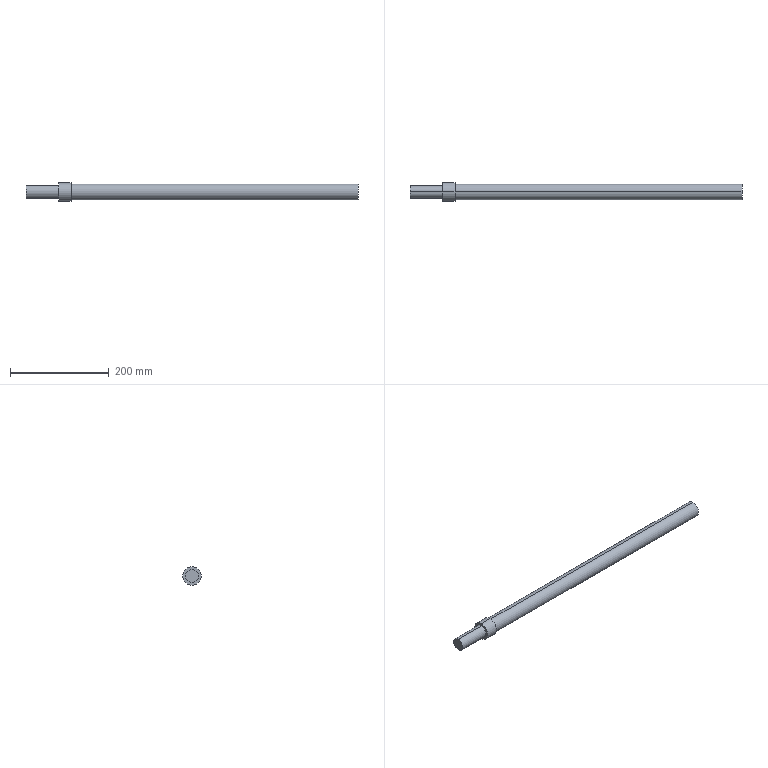Part | SolidWorks | features Revolution 1 | 1 solid | 10 faces | box 671 x 37 x 37 mm | volume 528385 mm3 | cylinder 6 | plane 4 | commonest cylinder face diameters 26 x2 32 x2 37 x2
STEP:
#1=CARTESIAN_POINT('',(589.602,0.,16.));
#2=VERTEX_POINT('',#1);
#3=CARTESIAN_POINT('',(589.602,0.,-16.));
#4=VERTEX_POINT('',#3);
#5=CARTESIAN_POINT('',(589.602,0.,0.));
#6=DIRECTION('',(-1.,0.,0.));
#7=DIRECTION('',(0.,0.,1.));
#8=AXIS2_PLACEMENT_3D('',#5,#6,#7);
#9=CIRCLE('',#8,16.);
#10=EDGE_CURVE('',#2,#4,#9,.T.);
#11=ORIENTED_EDGE('',*,*,#10,.T.);
#12=CARTESIAN_POINT('',(9.602,0.,-16.));
#13=VERTEX_POINT('',#12);
#14=CARTESIAN_POINT('',(-87.303,0.,-16.));
#15=DIRECTION('',(-1.,0.,0.));
#16=VECTOR('',#15,1000.);
#17=LINE('',#14,#16);
#18=EDGE_CURVE('',#4,#13,#17,.T.);
#19=ORIENTED_EDGE('',*,*,#18,.T.);
#20=CARTESIAN_POINT('',(9.602,0.,16.));
#21=VERTEX_POINT('',#20);
#22=CARTESIAN_POINT('',(9.602,0.,0.));
#23=DIRECTION('',(-1.,0.,0.));
#24=DIRECTION('',(0.,0.,1.));
#25=AXIS2_PLACEMENT_3D('',#22,#23,#24);
#26=CIRCLE('',#25,16.);
#27=EDGE_CURVE('',#21,#13,#26,.T.);
#28=ORIENTED_EDGE('',*,*,#27,.F.);
#29=CARTESIAN_POINT('',(-87.303,0.,16.));
#30=DIRECTION('',(-1.,0.,0.));
#31=VECTOR('',#30,1000.);
#32=LINE('',#29,#31);
#33=EDGE_CURVE('',#2,#21,#32,.T.);
#34=ORIENTED_EDGE('',*,*,#33,.F.);
#35=EDGE_LOOP('',(#11,#19,#28,#34));
#36=FACE_OUTER_BOUND('',#35,.T.);
#37=CARTESIAN_POINT('',(-87.303,0.,0.));
#38=DIRECTION('',(-1.,0.,0.));
#39=DIRECTION('',(0.,0.,1.));
#40=AXIS2_PLACEMENT_3D('',#37,#38,#39);
#41=CYLINDRICAL_SURFACE('',#40,16.);
#42=ADVANCED_FACE('',(#36),#41,.T.);
#43=CARTESIAN_POINT('',(9.602,0.,18.5));
#44=VERTEX_POINT('',#43);
#45=CARTESIAN_POINT('',(9.602,0.,-18.5));
#46=VERTEX_POINT('',#45);
#47=CARTESIAN_POINT('',(9.602,0.,0.));
#48=DIRECTION('',(-1.,0.,0.));
#49=DIRECTION('',(0.,0.,1.));
#50=AXIS2_PLACEMENT_3D('',#47,#48,#49);
#51=CIRCLE('',#50,18.5);
#52=EDGE_CURVE('',#44,#46,#51,.T.);
#53=ORIENTED_EDGE('',*,*,#52,.T.);
#54=CARTESIAN_POINT('',(-15.398,0.,-18.5));
#55=VERTEX_POINT('',#54);
#56=CARTESIAN_POINT('',(-87.303,0.,-18.5));
#57=DIRECTION('',(-1.,0.,0.));
#58=VECTOR('',#57,1000.);
#59=LINE('',#56,#58);
#60=EDGE_CURVE('',#46,#55,#59,.T.);
#61=ORIENTED_EDGE('',*,*,#60,.T.);
#62=CARTESIAN_POINT('',(-15.398,0.,18.5));
#63=VERTEX_POINT('',#62);
#64=CARTESIAN_POINT('',(-15.398,0.,0.));
#65=DIRECTION('',(-1.,0.,0.));
#66=DIRECTION('',(0.,0.,1.));
#67=AXIS2_PLACEMENT_3D('',#64,#65,#66);
#68=CIRCLE('',#67,18.5);
#69=EDGE_CURVE('',#63,#55,#68,.T.);
#70=ORIENTED_EDGE('',*,*,#69,.F.);
#71=CARTESIAN_POINT('',(-87.303,0.,18.5));
#72=DIRECTION('',(-1.,0.,0.));
#73=VECTOR('',#72,1000.);
#74=LINE('',#71,#73);
#75=EDGE_CURVE('',#44,#63,#74,.T.);
#76=ORIENTED_EDGE('',*,*,#75,.F.);
#77=EDGE_LOOP('',(#53,#61,#70,#76));
#78=FACE_OUTER_BOUND('',#77,.T.);
#79=CARTESIAN_POINT('',(-87.303,0.,0.));
#80=DIRECTION('',(-1.,0.,0.));
#81=DIRECTION('',(0.,0.,1.));
#82=AXIS2_PLACEMENT_3D('',#79,#80,#81);
#83=CYLINDRICAL_SURFACE('',#82,18.5);
#84=ADVANCED_FACE('',(#78),#83,.T.);
#85=CARTESIAN_POINT('',(-15.398,0.,13.));
#86=VERTEX_POINT('',#85);
#87=CARTESIAN_POINT('',(-15.398,0.,-13.));
#88=VERTEX_POINT('',#87);
#89=CARTESIAN_POINT('',(-15.398,0.,0.));
#90=DIRECTION('',(-1.,0.,0.));
#91=DIRECTION('',(0.,0.,1.));
#92=AXIS2_PLACEMENT_3D('',#89,#90,#91);
#93=CIRCLE('',#92,13.);
#94=EDGE_CURVE('',#86,#88,#93,.T.);
#95=ORIENTED_EDGE('',*,*,#94,.T.);
#96=CARTESIAN_POINT('',(-81.398,0.,-13.));
#97=VERTEX_POINT('',#96);
#98=CARTESIAN_POINT('',(-87.303,0.,-13.));
#99=DIRECTION('',(-1.,0.,0.));
#100=VECTOR('',#99,1000.);
#101=LINE('',#98,#100);
#102=EDGE_CURVE('',#88,#97,#101,.T.);
#103=ORIENTED_EDGE('',*,*,#102,.T.);
#104=CARTESIAN_POINT('',(-81.398,0.,13.));
#105=VERTEX_POINT('',#104);
#106=CARTESIAN_POINT('',(-81.398,0.,0.));
#107=DIRECTION('',(-1.,0.,0.));
#108=DIRECTION('',(0.,0.,1.));
#109=AXIS2_PLACEMENT_3D('',#106,#107,#108);
#110=CIRCLE('',#109,13.);
#111=EDGE_CURVE('',#105,#97,#110,.T.);
#112=ORIENTED_EDGE('',*,*,#111,.F.);
#113=CARTESIAN_POINT('',(-87.303,0.,13.));
#114=DIRECTION('',(-1.,0.,0.));
#115=VECTOR('',#114,1000.);
#116=LINE('',#113,#115);
#117=EDGE_CURVE('',#86,#105,#116,.T.);
#118=ORIENTED_EDGE('',*,*,#117,.F.);
#119=EDGE_LOOP('',(#95,#103,#112,#118));
#120=FACE_OUTER_BOUND('',#119,.T.);
#121=CARTESIAN_POINT('',(-87.303,0.,0.));
#122=DIRECTION('',(-1.,0.,0.));
#123=DIRECTION('',(0.,0.,1.));
#124=AXIS2_PLACEMENT_3D('',#121,#122,#123);
#125=CYLINDRICAL_SURFACE('',#124,13.);
#126=ADVANCED_FACE('',(#120),#125,.T.);
#127=ORIENTED_EDGE('',*,*,#111,.T.);
#128=CARTESIAN_POINT('',(-81.398,0.,0.));
#129=DIRECTION('',(-1.,0.,0.));
#130=DIRECTION('',(0.,0.,1.));
#131=AXIS2_PLACEMENT_3D('',#128,#129,#130);
#132=CIRCLE('',#131,13.);
#133=EDGE_CURVE('',#97,#105,#132,.T.);
#134=ORIENTED_EDGE('',*,*,#133,.T.);
#135=EDGE_LOOP('',(#127,#134));
#136=FACE_OUTER_BOUND('',#135,.T.);
#137=CARTESIAN_POINT('',(-81.398,0.,0.));
#138=DIRECTION('',(1.,0.,0.));
#139=DIRECTION('',(0.,0.,-1.));
#140=AXIS2_PLACEMENT_3D('',#137,#138,#139);
#141=PLANE('',#140);
#142=ADVANCED_FACE('',(#136),#141,.F.);
#143=ORIENTED_EDGE('',*,*,#102,.F.);
#144=CARTESIAN_POINT('',(-15.398,0.,0.));
#145=DIRECTION('',(-1.,0.,0.));
#146=DIRECTION('',(0.,0.,1.));
#147=AXIS2_PLACEMENT_3D('',#144,#145,#146);
#148=CIRCLE('',#147,13.);
#149=EDGE_CURVE('',#88,#86,#148,.T.);
#150=ORIENTED_EDGE('',*,*,#149,.T.);
#151=ORIENTED_EDGE('',*,*,#117,.T.);
#152=ORIENTED_EDGE('',*,*,#133,.F.);
#153=EDGE_LOOP('',(#143,#150,#151,#152));
#154=FACE_OUTER_BOUND('',#153,.T.);
#155=CARTESIAN_POINT('',(-87.303,0.,0.));
#156=DIRECTION('',(-1.,0.,0.));
#157=DIRECTION('',(0.,0.,1.));
#158=AXIS2_PLACEMENT_3D('',#155,#156,#157);
#159=CYLINDRICAL_SURFACE('',#158,13.);
#160=ADVANCED_FACE('',(#154),#159,.T.);
#161=ORIENTED_EDGE('',*,*,#94,.F.);
#162=ORIENTED_EDGE('',*,*,#149,.F.);
#163=EDGE_LOOP('',(#161,#162));
#164=FACE_BOUND('',#163,.T.);
#165=ORIENTED_EDGE('',*,*,#69,.T.);
#166=CARTESIAN_POINT('',(-15.398,0.,0.));
#167=DIRECTION('',(-1.,0.,0.));
#168=DIRECTION('',(0.,0.,1.));
#169=AXIS2_PLACEMENT_3D('',#166,#167,#168);
#170=CIRCLE('',#169,18.5);
#171=EDGE_CURVE('',#55,#63,#170,.T.);
#172=ORIENTED_EDGE('',*,*,#171,.T.);
#173=EDGE_LOOP('',(#165,#172));
#174=FACE_OUTER_BOUND('',#173,.T.);
#175=CARTESIAN_POINT('',(-15.398,13.,0.));
#176=DIRECTION('',(1.,0.,0.));
#177=DIRECTION('',(0.,0.,-1.));
#178=AXIS2_PLACEMENT_3D('',#175,#176,#177);
#179=PLANE('',#178);
#180=ADVANCED_FACE('',(#164,#174),#179,.F.);
#181=ORIENTED_EDGE('',*,*,#60,.F.);
#182=CARTESIAN_POINT('',(9.602,0.,0.));
#183=DIRECTION('',(-1.,0.,0.));
#184=DIRECTION('',(0.,0.,1.));
#185=AXIS2_PLACEMENT_3D('',#182,#183,#184);
#186=CIRCLE('',#185,18.5);
#187=EDGE_CURVE('',#46,#44,#186,.T.);
#188=ORIENTED_EDGE('',*,*,#187,.T.);
#189=ORIENTED_EDGE('',*,*,#75,.T.);
#190=ORIENTED_EDGE('',*,*,#171,.F.);
#191=EDGE_LOOP('',(#181,#188,#189,#190));
#192=FACE_OUTER_BOUND('',#191,.T.);
#193=CARTESIAN_POINT('',(-87.303,0.,0.));
#194=DIRECTION('',(-1.,0.,0.));
#195=DIRECTION('',(0.,0.,1.));
#196=AXIS2_PLACEMENT_3D('',#193,#194,#195);
#197=CYLINDRICAL_SURFACE('',#196,18.5);
#198=ADVANCED_FACE('',(#192),#197,.T.);
#199=ORIENTED_EDGE('',*,*,#52,.F.);
#200=ORIENTED_EDGE('',*,*,#187,.F.);
#201=EDGE_LOOP('',(#199,#200));
#202=FACE_OUTER_BOUND('',#201,.T.);
#203=ORIENTED_EDGE('',*,*,#27,.T.);
#204=CARTESIAN_POINT('',(9.602,0.,0.));
#205=DIRECTION('',(-1.,0.,0.));
#206=DIRECTION('',(0.,0.,1.));
#207=AXIS2_PLACEMENT_3D('',#204,#205,#206);
#208=CIRCLE('',#207,16.);
#209=EDGE_CURVE('',#13,#21,#208,.T.);
#210=ORIENTED_EDGE('',*,*,#209,.T.);
#211=EDGE_LOOP('',(#203,#210));
#212=FACE_BOUND('',#211,.T.);
#213=CARTESIAN_POINT('',(9.602,18.5,0.));
#214=DIRECTION('',(-1.,0.,0.));
#215=DIRECTION('',(0.,0.,1.));
#216=AXIS2_PLACEMENT_3D('',#213,#214,#215);
#217=PLANE('',#216);
#218=ADVANCED_FACE('',(#202,#212),#217,.F.);
#219=ORIENTED_EDGE('',*,*,#18,.F.);
#220=CARTESIAN_POINT('',(589.602,0.,0.));
#221=DIRECTION('',(-1.,0.,0.));
#222=DIRECTION('',(0.,0.,1.));
#223=AXIS2_PLACEMENT_3D('',#220,#221,#222);
#224=CIRCLE('',#223,16.);
#225=EDGE_CURVE('',#4,#2,#224,.T.);
#226=ORIENTED_EDGE('',*,*,#225,.T.);
#227=ORIENTED_EDGE('',*,*,#33,.T.);
#228=ORIENTED_EDGE('',*,*,#209,.F.);
#229=EDGE_LOOP('',(#219,#226,#227,#228));
#230=FACE_OUTER_BOUND('',#229,.T.);
#231=CARTESIAN_POINT('',(-87.303,0.,0.));
#232=DIRECTION('',(-1.,0.,0.));
#233=DIRECTION('',(0.,0.,1.));
#234=AXIS2_PLACEMENT_3D('',#231,#232,#233);
#235=CYLINDRICAL_SURFACE('',#234,16.);
#236=ADVANCED_FACE('',(#230),#235,.T.);
#237=ORIENTED_EDGE('',*,*,#10,.F.);
#238=ORIENTED_EDGE('',*,*,#225,.F.);
#239=EDGE_LOOP('',(#237,#238));
#240=FACE_OUTER_BOUND('',#239,.T.);
#241=CARTESIAN_POINT('',(589.602,16.,0.));
#242=DIRECTION('',(-1.,0.,0.));
#243=DIRECTION('',(0.,0.,1.));
#244=AXIS2_PLACEMENT_3D('',#241,#242,#243);
#245=PLANE('',#244);
#246=ADVANCED_FACE('',(#240),#245,.F.);
#247=CLOSED_SHELL('',(#42,#84,#126,#142,#160,#180,#198,#218,#236,#246));
#248=MANIFOLD_SOLID_BREP('',#247);
#249=CARTESIAN_POINT('',(0.,0.,0.));
#250=DIRECTION('',(0.,0.,1.));
#251=DIRECTION('',(1.,0.,0.));
#252=AXIS2_PLACEMENT_3D('',#249,#250,#251);
#253=(LENGTH_UNIT()NAMED_UNIT(*)SI_UNIT(.MILLI.,.METRE.));
#254=UNCERTAINTY_MEASURE_WITH_UNIT(LENGTH_MEASURE(0.00001),#253,'','');
#255=(NAMED_UNIT(*)PLANE_ANGLE_UNIT()SI_UNIT($,.RADIAN.));
#256=(NAMED_UNIT(*)SI_UNIT($,.STERADIAN.)SOLID_ANGLE_UNIT());
#257=(GEOMETRIC_REPRESENTATION_CONTEXT(3)GLOBAL_UNCERTAINTY_ASSIGNED_CONTEXT((#254))GLOBAL_UNIT_ASSIGNED_CONTEXT((#253,#255,#256))REPRESENTATION_CONTEXT('',''));
#258=ADVANCED_BREP_SHAPE_REPRESENTATION('',(#248,#252),#257);